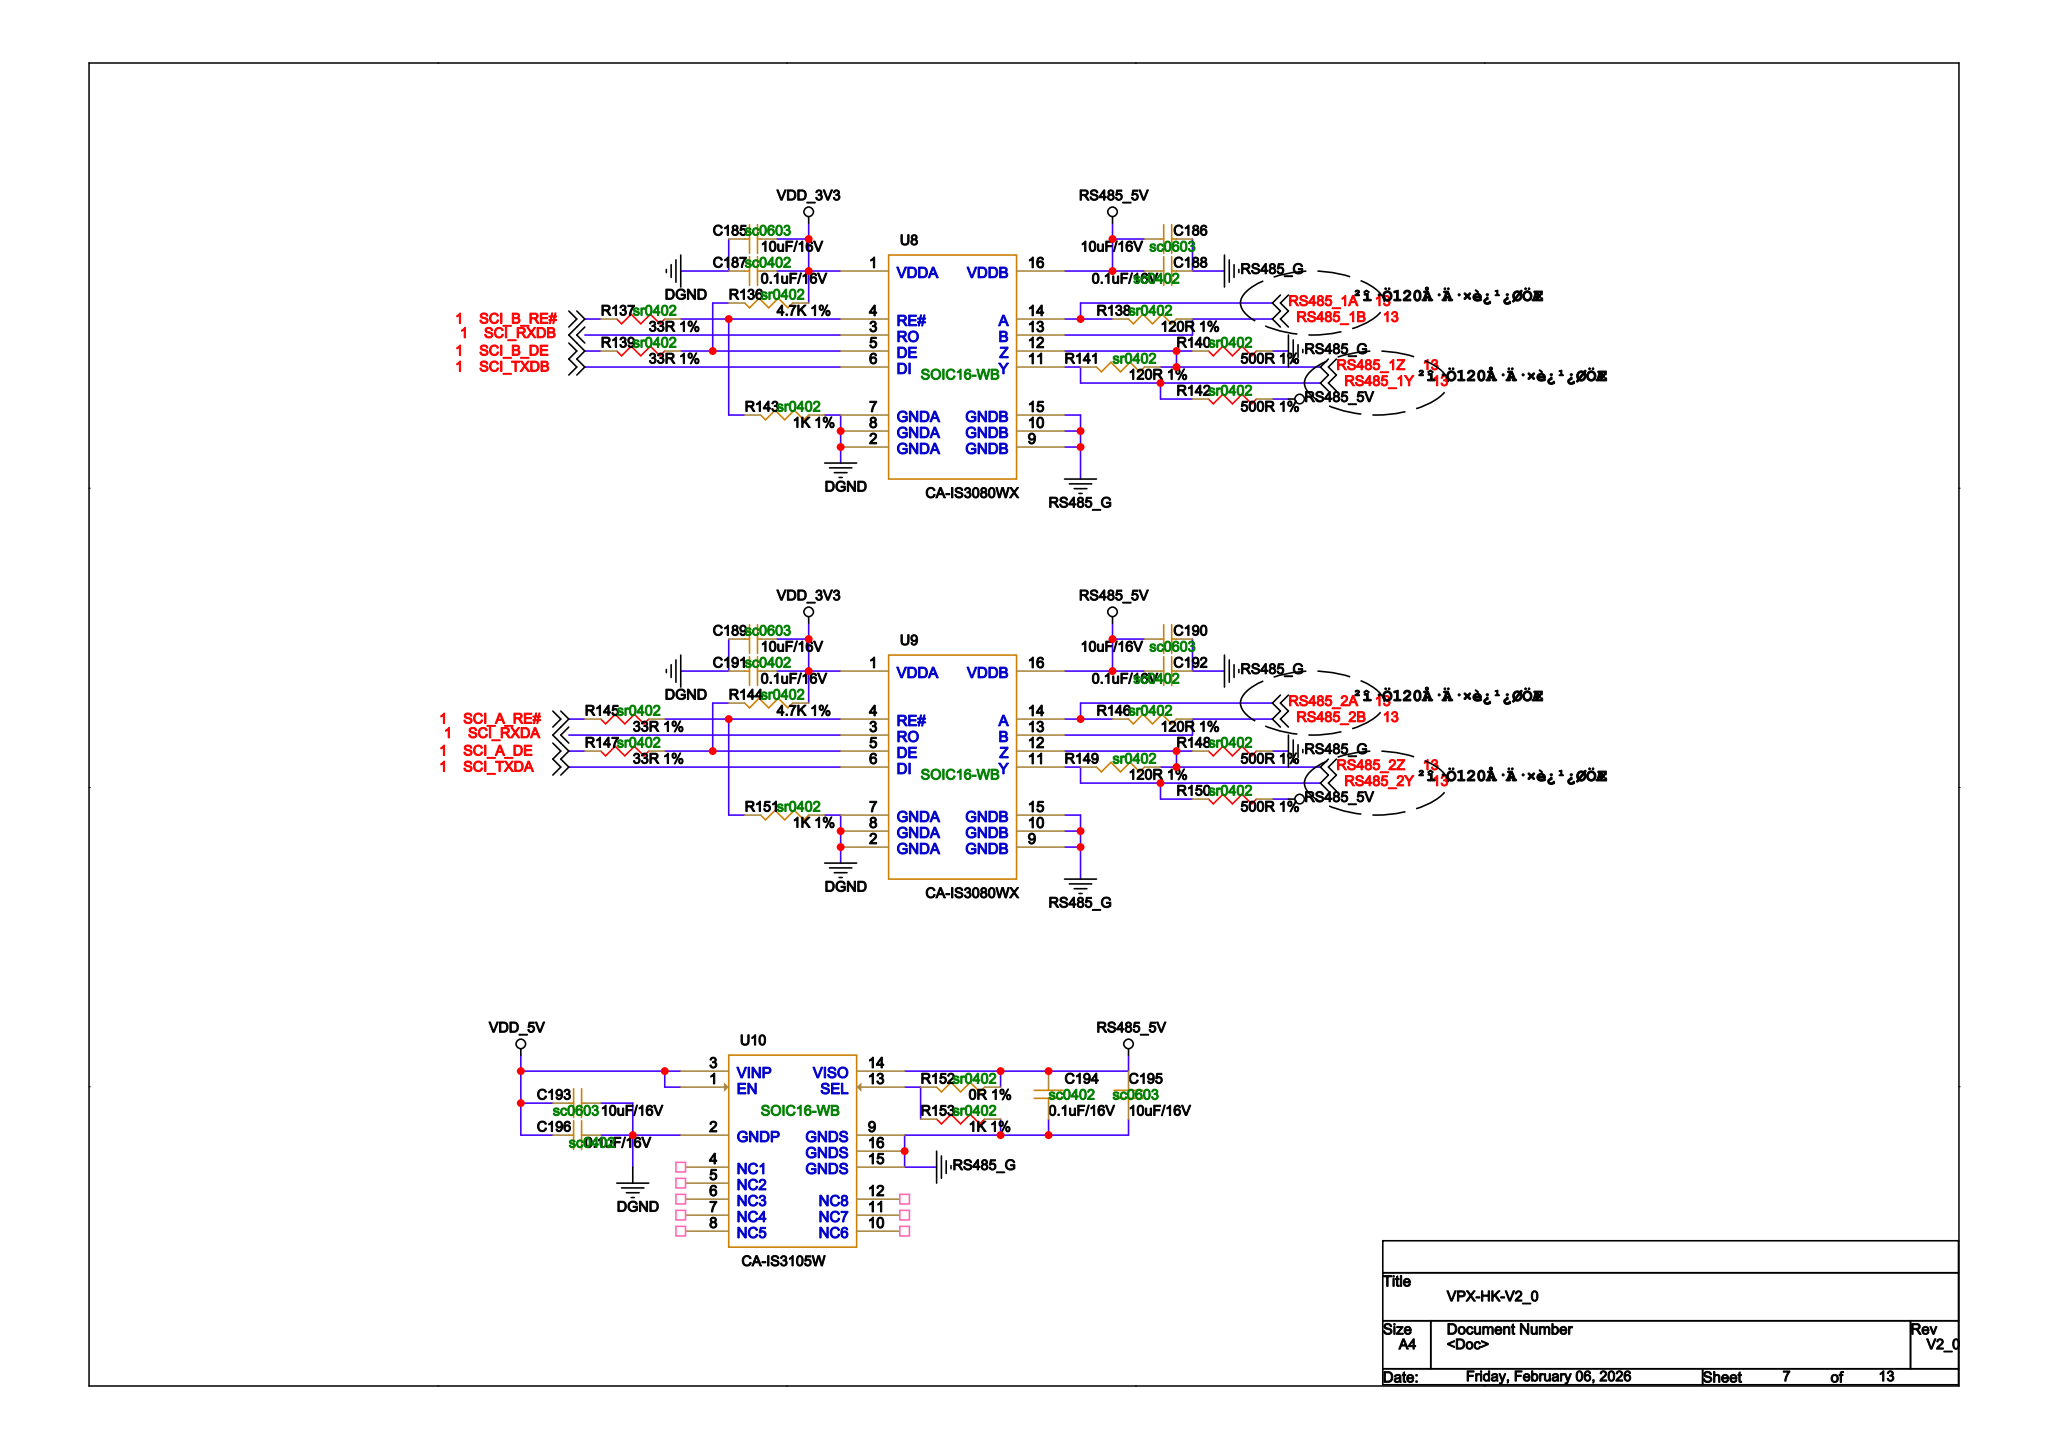Circuit board | Cadence Allegro | 598 parts | 541 nets | one sheet of the schematic
Parts on this sheet (reference | value | footprint):
C185 | 10uF/16V | SC0603
C186 | 10uF/16V | SC0603
C187 | 0.1uF/16V | SC0402
C188 | 0.1uF/16V | SC0402
C189 | 10uF/16V | SC0603
C190 | 10uF/16V | SC0603
C191 | 0.1uF/16V | SC0402
C192 | 0.1uF/16V | SC0402
C193 | 10uF/16V | SC0603
C194 | 0.1uF/16V | SC0402
C195 | 10uF/16V | SC0603
C196 | 0.1uF/16V | SC0402
R136 | 4.7K 1% | SR0402
R137 | 33R 1% | SR0402
R138 | 120R 1% | SR0402
R139 | 33R 1% | SR0402
R140 | 500R 1% | SR0402
R141 | 120R 1% | SR0402
R142 | 500R 1% | SR0402
R143 | 1K 1% | SR0402
R144 | 4.7K 1% | SR0402
R145 | 33R 1% | SR0402
R146 | 120R 1% | SR0402
R147 | 33R 1% | SR0402
R148 | 500R 1% | SR0402
R149 | 120R 1% | SR0402
R150 | 500R 1% | SR0402
R151 | 1K 1% | SR0402
R152 | 0R 1% | SR0402
R153 | 1K 1% | SR0402
U8 | CA-IS3080WX | SOIC16-WB
U9 | CA-IS3080WX | SOIC16-WB
U10 | CA-IS3105W | SOIC16-WB
Nets of these parts (net: part-pin ...):
DGND: C185-2 C187-2 C189-2 C191-2 C193-1 C196-1 R143-1 R151-1 U8-2 U8-7 U8-8 U9-2 U9-7 U9-8 U10-2
VDD_5V: C193-2 C196-2 U10-1 U10-3
VDD_3V3: C185-1 C187-1 C189-1 C191-1 R136-1 R144-1 U8-1 U9-1
RS485_5V: C186-1 C188-1 C190-1 C192-1 C194-1 C195-1 R142-2 R150-2 R152-1 U8-16 U9-16 U10-14
N33400995: R152-2 R153-2 U10-13
RS485_1Y: R141-1 R142-1 U8-11
RS485_1Z: R140-1 R141-2 U8-12
RS485_G: C186-2 C188-2 C190-2 C192-2 C194-2 C195-2 R140-2 R148-2 R153-1 U8-9 U8-10 U8-15 U9-9 U9-10 U9-15 U10-9 U10-15 U10-16
RS485_2Z: R148-1 R149-2 U9-12
RS485_2Y: R149-1 R150-1 U9-11
N32580796: R137-1 R143-2 U8-4
N33398545: R145-1 R151-2 U9-4
RS485_1A: R138-1 U8-14
RS485_1B: R138-2 U8-13
RS485_2A: R146-1 U9-14
RS485_2B: R146-2 U9-13
N32687242: R136-2 R139-1 U8-5
N33398786: R144-2 R147-1 U9-5
SCI_B_RE#: R137-2
SCI_B_DE: R139-2
SCI_A_RE#: R145-2
SCI_A_DE: R147-2
SCI_TXDB: U8-6
SCI_RXDB: U8-3
SCI_RXDA: U9-3
SCI_TXDA: U9-6